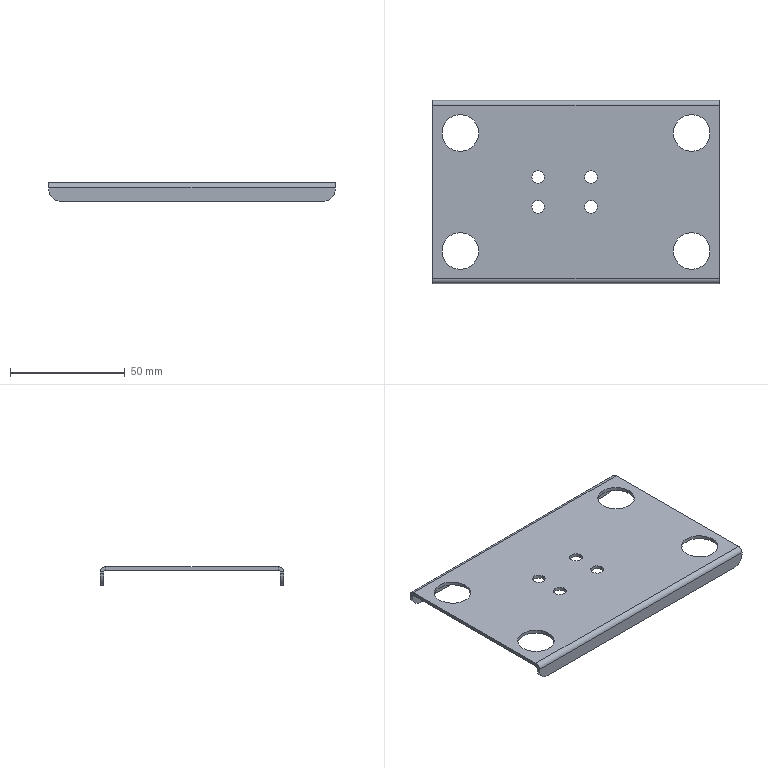Part | STEP file | A14-038 | 1 solid | 42 faces | box 125 x 80 x 8 mm | volume 15817 mm3 | cylinder 24 | plane 18 | commonest cylinder face diameters 5.5 x8 16 x8 10 x4 1.473 x2 4.473 x2